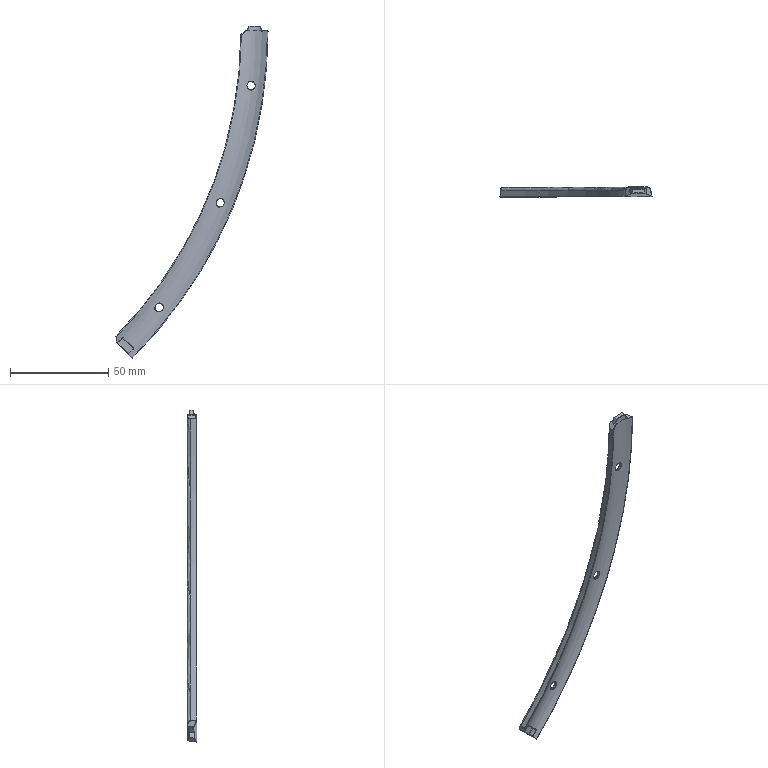Part | STEP file | 101000007695 | 1 solid | 178 faces | box 77.497 x 4.891 x 169.241 mm | volume 7806 mm3 | spline 58 | sphere 41 | cylinder 33 | plane 18 | torus 14 | cone 14 | commonest cylinder face diameters 0.4 x20 4.2 x6 8 x6 25.4 x1